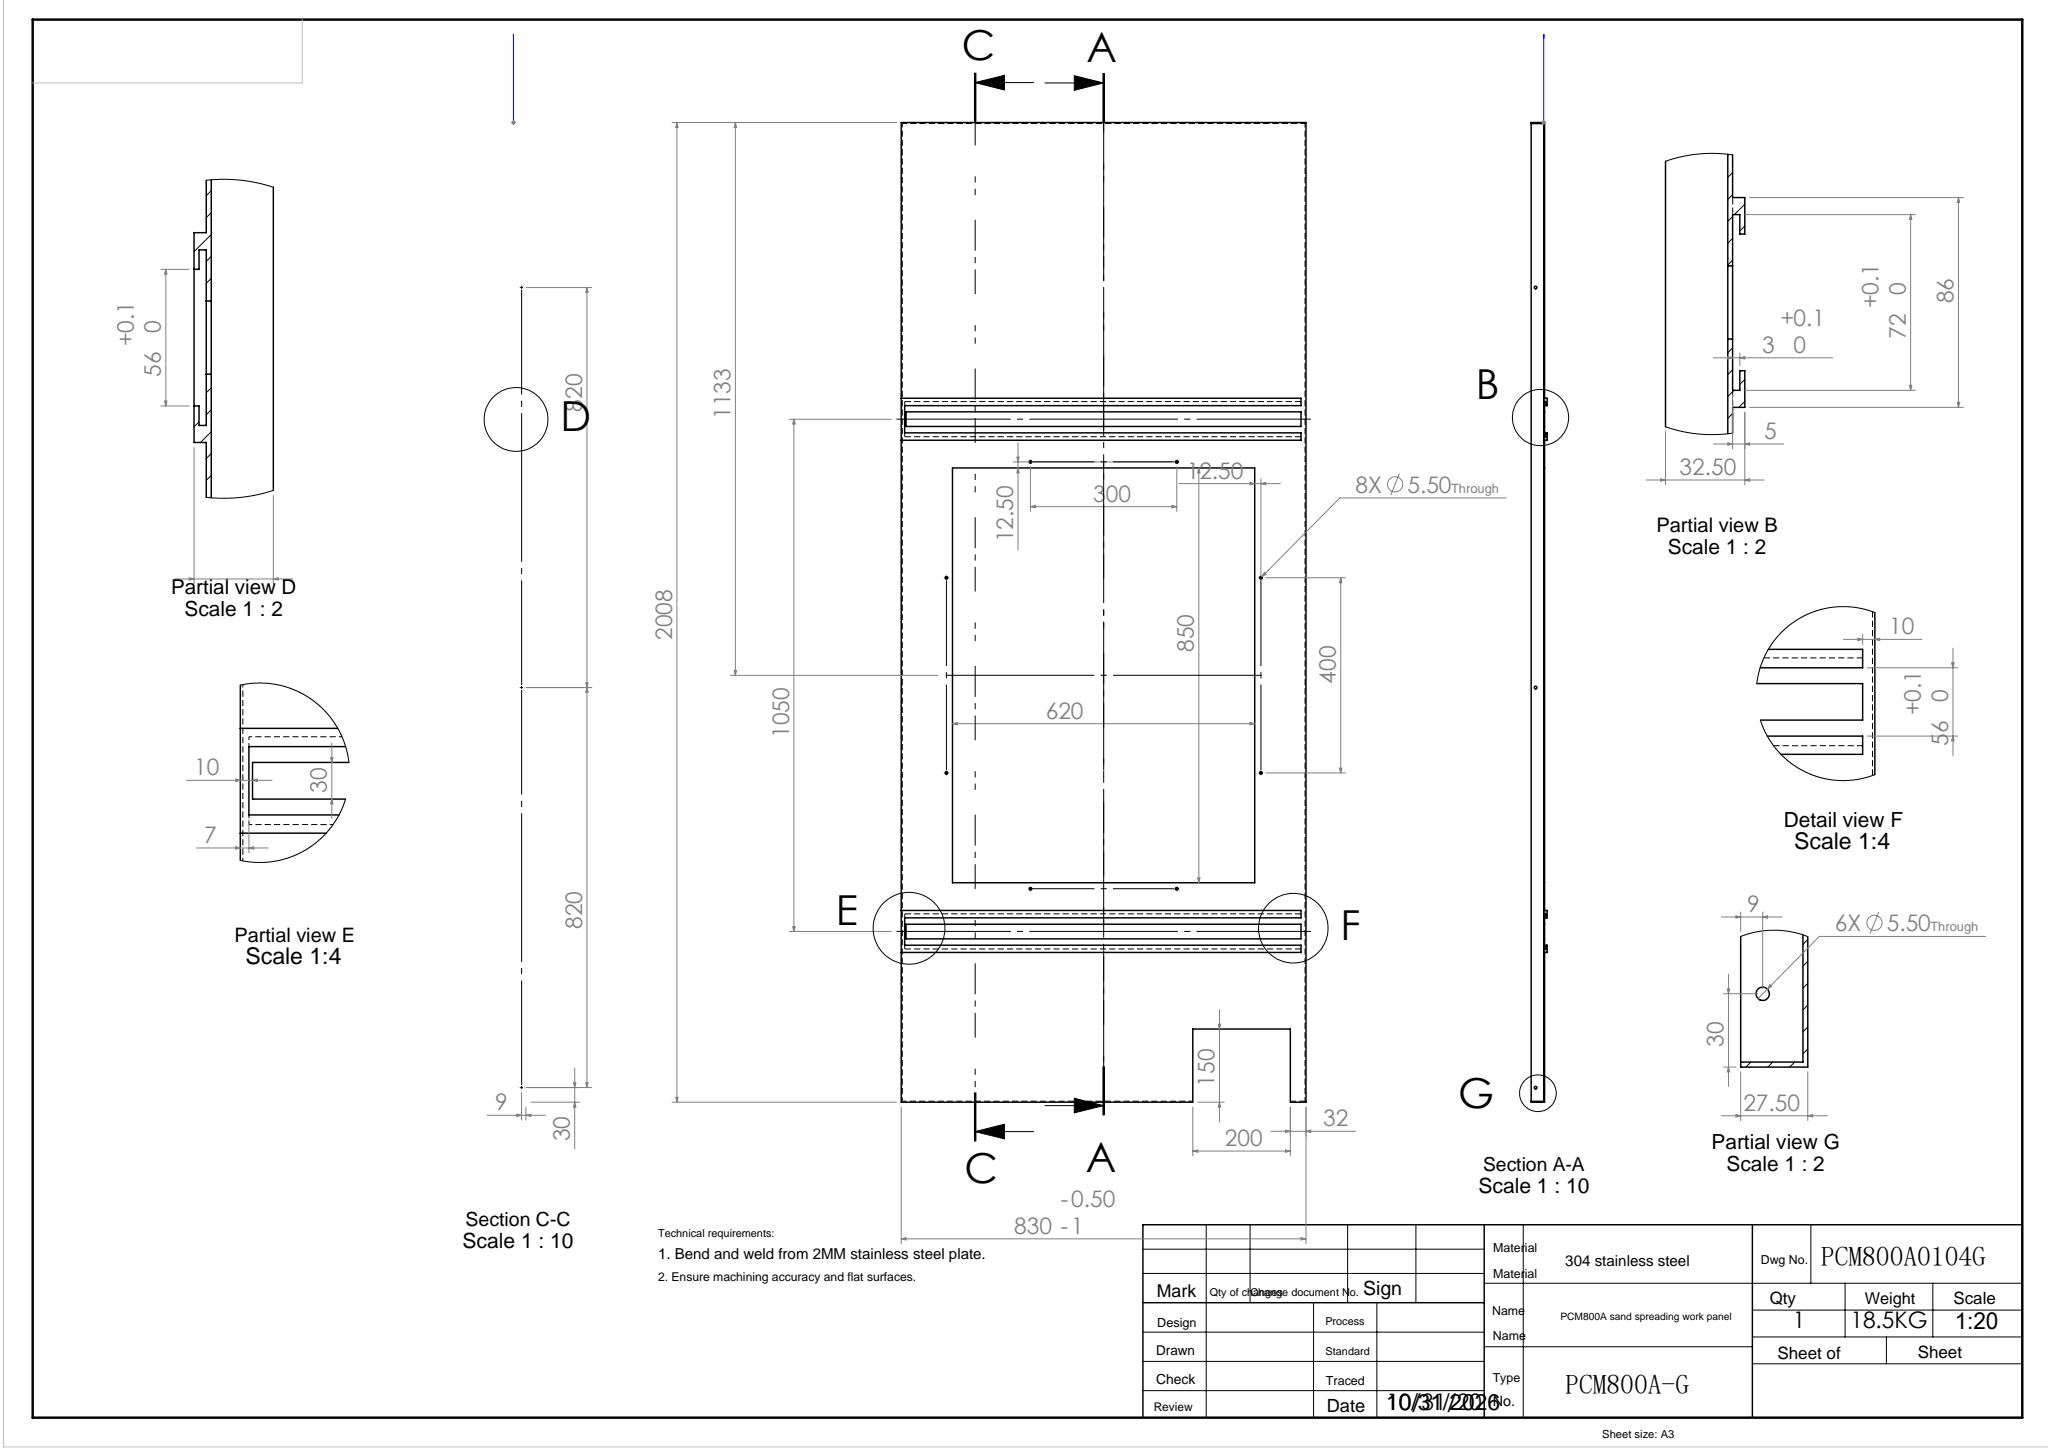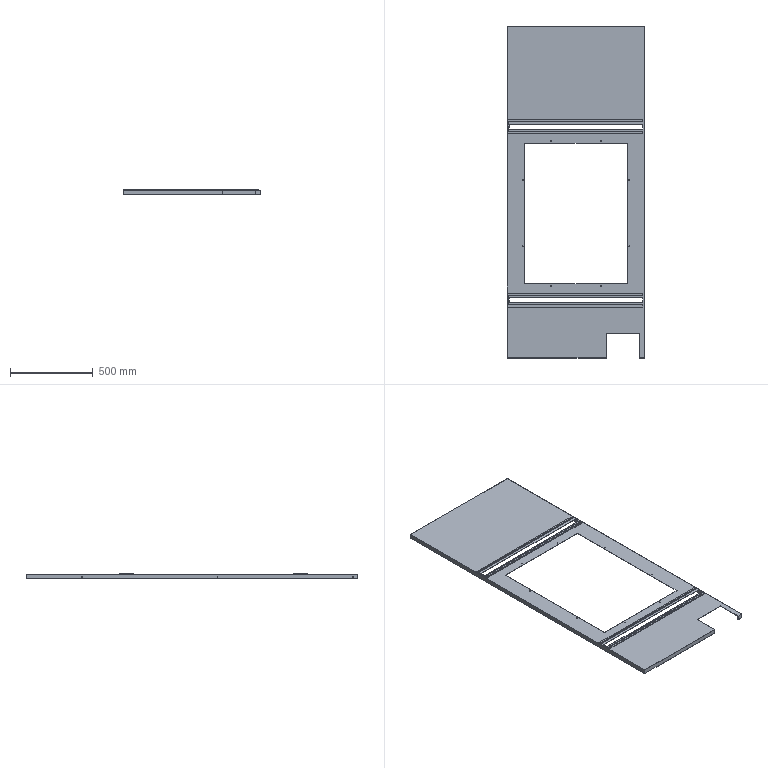Part | SolidWorks | features ICE 8, Extrusion 1, LPattern 1 | 1 solid | 80 faces | box 830 x 2008 x 32.5 mm | volume 2572177 mm3 | plane 52 | cylinder 28 | commonest cylinder face diameters 5.5 x28